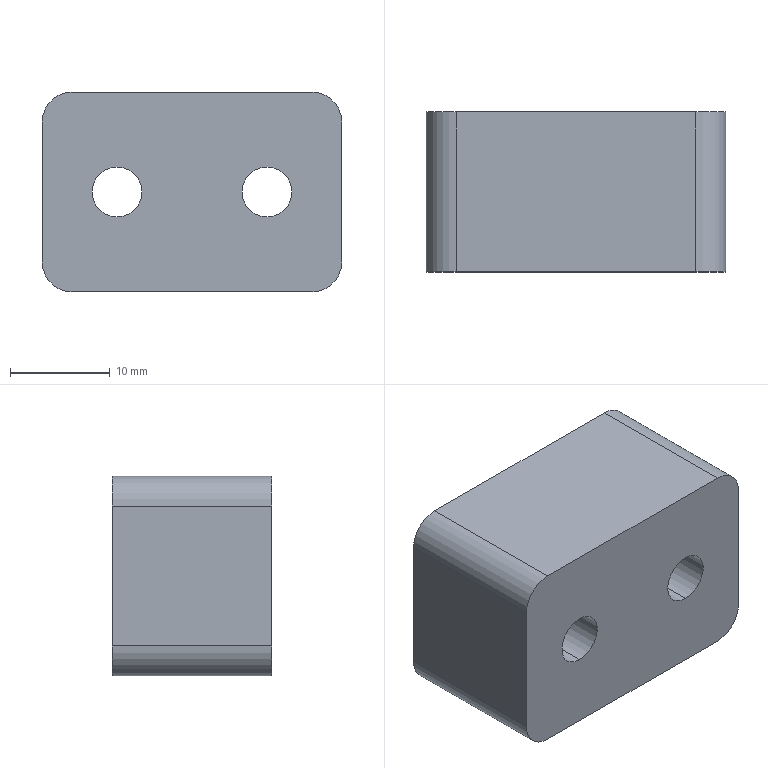Part | SolidWorks | features BaseBody 1 | 1 solid | 14 faces | box 30 x 16 x 20 mm | volume 8848 mm3 | cylinder 8 | plane 6 | commonest cylinder face diameters 5 x4 6 x4
STEP:
#1=CARTESIAN_POINT('',(-7.5,0.,-2.5));
#2=VERTEX_POINT('',#1);
#3=CARTESIAN_POINT('',(-7.5,0.,2.5));
#4=VERTEX_POINT('',#3);
#5=CARTESIAN_POINT('',(-7.5,0.,0.));
#6=DIRECTION('',(0.,1.,0.));
#7=DIRECTION('',(0.,0.,1.));
#8=AXIS2_PLACEMENT_3D('',#5,#6,#7);
#9=CIRCLE('',#8,2.5);
#10=EDGE_CURVE('',#2,#4,#9,.T.);
#11=ORIENTED_EDGE('',*,*,#10,.F.);
#12=CARTESIAN_POINT('',(-7.5,16.,-2.5));
#13=VERTEX_POINT('',#12);
#14=CARTESIAN_POINT('',(-7.5,0.,-2.5));
#15=DIRECTION('',(0.,1.,0.));
#16=VECTOR('',#15,1000.);
#17=LINE('',#14,#16);
#18=EDGE_CURVE('',#2,#13,#17,.T.);
#19=ORIENTED_EDGE('',*,*,#18,.T.);
#20=CARTESIAN_POINT('',(-7.5,16.,2.5));
#21=VERTEX_POINT('',#20);
#22=CARTESIAN_POINT('',(-7.5,16.,0.));
#23=DIRECTION('',(0.,-1.,0.));
#24=DIRECTION('',(0.,0.,1.));
#25=AXIS2_PLACEMENT_3D('',#22,#23,#24);
#26=CIRCLE('',#25,2.5);
#27=EDGE_CURVE('',#21,#13,#26,.T.);
#28=ORIENTED_EDGE('',*,*,#27,.F.);
#29=CARTESIAN_POINT('',(-7.5,0.,2.5));
#30=DIRECTION('',(0.,1.,0.));
#31=VECTOR('',#30,1000.);
#32=LINE('',#29,#31);
#33=EDGE_CURVE('',#4,#21,#32,.T.);
#34=ORIENTED_EDGE('',*,*,#33,.F.);
#35=EDGE_LOOP('',(#11,#19,#28,#34));
#36=FACE_OUTER_BOUND('',#35,.T.);
#37=CARTESIAN_POINT('',(-7.5,0.,0.));
#38=DIRECTION('',(0.,1.,0.));
#39=DIRECTION('',(0.,0.,1.));
#40=AXIS2_PLACEMENT_3D('',#37,#38,#39);
#41=CYLINDRICAL_SURFACE('',#40,2.5);
#42=ADVANCED_FACE('',(#36),#41,.F.);
#43=CARTESIAN_POINT('',(7.5,0.,-2.5));
#44=VERTEX_POINT('',#43);
#45=CARTESIAN_POINT('',(7.5,0.,2.5));
#46=VERTEX_POINT('',#45);
#47=CARTESIAN_POINT('',(7.5,0.,0.));
#48=DIRECTION('',(0.,1.,0.));
#49=DIRECTION('',(0.,0.,1.));
#50=AXIS2_PLACEMENT_3D('',#47,#48,#49);
#51=CIRCLE('',#50,2.5);
#52=EDGE_CURVE('',#44,#46,#51,.T.);
#53=ORIENTED_EDGE('',*,*,#52,.F.);
#54=CARTESIAN_POINT('',(7.5,16.,-2.5));
#55=VERTEX_POINT('',#54);
#56=CARTESIAN_POINT('',(7.5,0.,-2.5));
#57=DIRECTION('',(0.,1.,0.));
#58=VECTOR('',#57,1000.);
#59=LINE('',#56,#58);
#60=EDGE_CURVE('',#44,#55,#59,.T.);
#61=ORIENTED_EDGE('',*,*,#60,.T.);
#62=CARTESIAN_POINT('',(7.5,16.,2.5));
#63=VERTEX_POINT('',#62);
#64=CARTESIAN_POINT('',(7.5,16.,0.));
#65=DIRECTION('',(0.,-1.,0.));
#66=DIRECTION('',(0.,0.,1.));
#67=AXIS2_PLACEMENT_3D('',#64,#65,#66);
#68=CIRCLE('',#67,2.5);
#69=EDGE_CURVE('',#63,#55,#68,.T.);
#70=ORIENTED_EDGE('',*,*,#69,.F.);
#71=CARTESIAN_POINT('',(7.5,0.,2.5));
#72=DIRECTION('',(0.,1.,0.));
#73=VECTOR('',#72,1000.);
#74=LINE('',#71,#73);
#75=EDGE_CURVE('',#46,#63,#74,.T.);
#76=ORIENTED_EDGE('',*,*,#75,.F.);
#77=EDGE_LOOP('',(#53,#61,#70,#76));
#78=FACE_OUTER_BOUND('',#77,.T.);
#79=CARTESIAN_POINT('',(7.5,0.,0.));
#80=DIRECTION('',(0.,1.,0.));
#81=DIRECTION('',(0.,0.,1.));
#82=AXIS2_PLACEMENT_3D('',#79,#80,#81);
#83=CYLINDRICAL_SURFACE('',#82,2.5);
#84=ADVANCED_FACE('',(#78),#83,.F.);
#85=CARTESIAN_POINT('',(15.,0.,-7.));
#86=VERTEX_POINT('',#85);
#87=CARTESIAN_POINT('',(15.,0.,7.));
#88=VERTEX_POINT('',#87);
#89=CARTESIAN_POINT('',(15.,0.,0.));
#90=DIRECTION('',(0.,0.,1.));
#91=VECTOR('',#90,1000.);
#92=LINE('',#89,#91);
#93=EDGE_CURVE('',#86,#88,#92,.T.);
#94=ORIENTED_EDGE('',*,*,#93,.T.);
#95=CARTESIAN_POINT('',(12.,0.,10.));
#96=VERTEX_POINT('',#95);
#97=CARTESIAN_POINT('',(12.,0.,7.));
#98=DIRECTION('',(0.,-1.,0.));
#99=DIRECTION('',(0.,0.,-1.));
#100=AXIS2_PLACEMENT_3D('',#97,#98,#99);
#101=CIRCLE('',#100,3.);
#102=EDGE_CURVE('',#88,#96,#101,.T.);
#103=ORIENTED_EDGE('',*,*,#102,.T.);
#104=CARTESIAN_POINT('',(-12.,0.,10.));
#105=VERTEX_POINT('',#104);
#106=CARTESIAN_POINT('',(0.,0.,10.));
#107=DIRECTION('',(-1.,0.,0.));
#108=VECTOR('',#107,1000.);
#109=LINE('',#106,#108);
#110=EDGE_CURVE('',#96,#105,#109,.T.);
#111=ORIENTED_EDGE('',*,*,#110,.T.);
#112=CARTESIAN_POINT('',(-15.,0.,7.));
#113=VERTEX_POINT('',#112);
#114=CARTESIAN_POINT('',(-12.,0.,7.));
#115=DIRECTION('',(0.,-1.,0.));
#116=DIRECTION('',(0.,0.,-1.));
#117=AXIS2_PLACEMENT_3D('',#114,#115,#116);
#118=CIRCLE('',#117,3.);
#119=EDGE_CURVE('',#105,#113,#118,.T.);
#120=ORIENTED_EDGE('',*,*,#119,.T.);
#121=CARTESIAN_POINT('',(-15.,0.,-7.));
#122=VERTEX_POINT('',#121);
#123=CARTESIAN_POINT('',(-15.,0.,0.));
#124=DIRECTION('',(0.,0.,-1.));
#125=VECTOR('',#124,1000.);
#126=LINE('',#123,#125);
#127=EDGE_CURVE('',#113,#122,#126,.T.);
#128=ORIENTED_EDGE('',*,*,#127,.T.);
#129=CARTESIAN_POINT('',(-12.,0.,-10.));
#130=VERTEX_POINT('',#129);
#131=CARTESIAN_POINT('',(-12.,0.,-7.));
#132=DIRECTION('',(0.,-1.,0.));
#133=DIRECTION('',(0.,0.,-1.));
#134=AXIS2_PLACEMENT_3D('',#131,#132,#133);
#135=CIRCLE('',#134,3.);
#136=EDGE_CURVE('',#122,#130,#135,.T.);
#137=ORIENTED_EDGE('',*,*,#136,.T.);
#138=CARTESIAN_POINT('',(12.,0.,-10.));
#139=VERTEX_POINT('',#138);
#140=CARTESIAN_POINT('',(0.,0.,-10.));
#141=DIRECTION('',(1.,0.,0.));
#142=VECTOR('',#141,1000.);
#143=LINE('',#140,#142);
#144=EDGE_CURVE('',#130,#139,#143,.T.);
#145=ORIENTED_EDGE('',*,*,#144,.T.);
#146=CARTESIAN_POINT('',(12.,0.,-7.));
#147=DIRECTION('',(0.,-1.,0.));
#148=DIRECTION('',(0.,0.,-1.));
#149=AXIS2_PLACEMENT_3D('',#146,#147,#148);
#150=CIRCLE('',#149,3.);
#151=EDGE_CURVE('',#139,#86,#150,.T.);
#152=ORIENTED_EDGE('',*,*,#151,.T.);
#153=EDGE_LOOP('',(#94,#103,#111,#120,#128,#137,#145,#152));
#154=FACE_OUTER_BOUND('',#153,.T.);
#155=CARTESIAN_POINT('',(-7.5,0.,0.));
#156=DIRECTION('',(0.,1.,0.));
#157=DIRECTION('',(0.,0.,1.));
#158=AXIS2_PLACEMENT_3D('',#155,#156,#157);
#159=CIRCLE('',#158,2.5);
#160=EDGE_CURVE('',#4,#2,#159,.T.);
#161=ORIENTED_EDGE('',*,*,#160,.T.);
#162=ORIENTED_EDGE('',*,*,#10,.T.);
#163=EDGE_LOOP('',(#161,#162));
#164=FACE_BOUND('',#163,.T.);
#165=CARTESIAN_POINT('',(7.5,0.,0.));
#166=DIRECTION('',(0.,1.,0.));
#167=DIRECTION('',(0.,0.,1.));
#168=AXIS2_PLACEMENT_3D('',#165,#166,#167);
#169=CIRCLE('',#168,2.5);
#170=EDGE_CURVE('',#46,#44,#169,.T.);
#171=ORIENTED_EDGE('',*,*,#170,.T.);
#172=ORIENTED_EDGE('',*,*,#52,.T.);
#173=EDGE_LOOP('',(#171,#172));
#174=FACE_BOUND('',#173,.T.);
#175=CARTESIAN_POINT('',(0.,0.,0.));
#176=DIRECTION('',(0.,-1.,0.));
#177=DIRECTION('',(0.,0.,-1.));
#178=AXIS2_PLACEMENT_3D('',#175,#176,#177);
#179=PLANE('',#178);
#180=ADVANCED_FACE('',(#154,#164,#174),#179,.T.);
#181=ORIENTED_EDGE('',*,*,#102,.F.);
#182=CARTESIAN_POINT('',(15.,16.,7.));
#183=VERTEX_POINT('',#182);
#184=CARTESIAN_POINT('',(15.,16.,7.));
#185=DIRECTION('',(0.,1.,0.));
#186=VECTOR('',#185,1000.);
#187=LINE('',#184,#186);
#188=EDGE_CURVE('',#88,#183,#187,.T.);
#189=ORIENTED_EDGE('',*,*,#188,.T.);
#190=CARTESIAN_POINT('',(12.,16.,10.));
#191=VERTEX_POINT('',#190);
#192=CARTESIAN_POINT('',(12.,16.,7.));
#193=DIRECTION('',(0.,-1.,0.));
#194=DIRECTION('',(0.,0.,-1.));
#195=AXIS2_PLACEMENT_3D('',#192,#193,#194);
#196=CIRCLE('',#195,3.);
#197=EDGE_CURVE('',#183,#191,#196,.T.);
#198=ORIENTED_EDGE('',*,*,#197,.T.);
#199=CARTESIAN_POINT('',(12.,16.,10.));
#200=DIRECTION('',(0.,-1.,0.));
#201=VECTOR('',#200,1000.);
#202=LINE('',#199,#201);
#203=EDGE_CURVE('',#191,#96,#202,.T.);
#204=ORIENTED_EDGE('',*,*,#203,.T.);
#205=EDGE_LOOP('',(#181,#189,#198,#204));
#206=FACE_OUTER_BOUND('',#205,.T.);
#207=CARTESIAN_POINT('',(12.,16.,7.));
#208=DIRECTION('',(0.,-1.,0.));
#209=DIRECTION('',(0.,0.,-1.));
#210=AXIS2_PLACEMENT_3D('',#207,#208,#209);
#211=CYLINDRICAL_SURFACE('',#210,3.);
#212=ADVANCED_FACE('',(#206),#211,.T.);
#213=CARTESIAN_POINT('',(15.,16.,-7.));
#214=VERTEX_POINT('',#213);
#215=CARTESIAN_POINT('',(15.,16.,-7.));
#216=DIRECTION('',(0.,-1.,0.));
#217=VECTOR('',#216,1000.);
#218=LINE('',#215,#217);
#219=EDGE_CURVE('',#214,#86,#218,.T.);
#220=ORIENTED_EDGE('',*,*,#219,.F.);
#221=CARTESIAN_POINT('',(15.,16.,10.));
#222=DIRECTION('',(0.,0.,-1.));
#223=VECTOR('',#222,1000.);
#224=LINE('',#221,#223);
#225=EDGE_CURVE('',#183,#214,#224,.T.);
#226=ORIENTED_EDGE('',*,*,#225,.F.);
#227=ORIENTED_EDGE('',*,*,#188,.F.);
#228=ORIENTED_EDGE('',*,*,#93,.F.);
#229=EDGE_LOOP('',(#220,#226,#227,#228));
#230=FACE_OUTER_BOUND('',#229,.T.);
#231=CARTESIAN_POINT('',(15.,16.,10.));
#232=DIRECTION('',(-1.,0.,0.));
#233=DIRECTION('',(0.,0.,1.));
#234=AXIS2_PLACEMENT_3D('',#231,#232,#233);
#235=PLANE('',#234);
#236=ADVANCED_FACE('',(#230),#235,.F.);
#237=ORIENTED_EDGE('',*,*,#151,.F.);
#238=CARTESIAN_POINT('',(12.,16.,-10.));
#239=VERTEX_POINT('',#238);
#240=CARTESIAN_POINT('',(12.,16.,-10.));
#241=DIRECTION('',(0.,1.,0.));
#242=VECTOR('',#241,1000.);
#243=LINE('',#240,#242);
#244=EDGE_CURVE('',#139,#239,#243,.T.);
#245=ORIENTED_EDGE('',*,*,#244,.T.);
#246=CARTESIAN_POINT('',(12.,16.,-7.));
#247=DIRECTION('',(0.,-1.,0.));
#248=DIRECTION('',(0.,0.,-1.));
#249=AXIS2_PLACEMENT_3D('',#246,#247,#248);
#250=CIRCLE('',#249,3.);
#251=EDGE_CURVE('',#239,#214,#250,.T.);
#252=ORIENTED_EDGE('',*,*,#251,.T.);
#253=ORIENTED_EDGE('',*,*,#219,.T.);
#254=EDGE_LOOP('',(#237,#245,#252,#253));
#255=FACE_OUTER_BOUND('',#254,.T.);
#256=CARTESIAN_POINT('',(12.,16.,-7.));
#257=DIRECTION('',(0.,-1.,0.));
#258=DIRECTION('',(0.,0.,-1.));
#259=AXIS2_PLACEMENT_3D('',#256,#257,#258);
#260=CYLINDRICAL_SURFACE('',#259,3.);
#261=ADVANCED_FACE('',(#255),#260,.T.);
#262=CARTESIAN_POINT('',(-12.,16.,-10.));
#263=VERTEX_POINT('',#262);
#264=CARTESIAN_POINT('',(-12.,16.,-10.));
#265=DIRECTION('',(0.,-1.,0.));
#266=VECTOR('',#265,1000.);
#267=LINE('',#264,#266);
#268=EDGE_CURVE('',#263,#130,#267,.T.);
#269=ORIENTED_EDGE('',*,*,#268,.F.);
#270=CARTESIAN_POINT('',(-15.,16.,-10.));
#271=DIRECTION('',(-1.,0.,0.));
#272=VECTOR('',#271,1000.);
#273=LINE('',#270,#272);
#274=EDGE_CURVE('',#239,#263,#273,.T.);
#275=ORIENTED_EDGE('',*,*,#274,.F.);
#276=ORIENTED_EDGE('',*,*,#244,.F.);
#277=ORIENTED_EDGE('',*,*,#144,.F.);
#278=EDGE_LOOP('',(#269,#275,#276,#277));
#279=FACE_OUTER_BOUND('',#278,.T.);
#280=CARTESIAN_POINT('',(-15.,16.,-10.));
#281=DIRECTION('',(0.,0.,1.));
#282=DIRECTION('',(1.,0.,0.));
#283=AXIS2_PLACEMENT_3D('',#280,#281,#282);
#284=PLANE('',#283);
#285=ADVANCED_FACE('',(#279),#284,.F.);
#286=ORIENTED_EDGE('',*,*,#136,.F.);
#287=CARTESIAN_POINT('',(-15.,16.,-7.));
#288=VERTEX_POINT('',#287);
#289=CARTESIAN_POINT('',(-15.,16.,-7.));
#290=DIRECTION('',(0.,1.,0.));
#291=VECTOR('',#290,1000.);
#292=LINE('',#289,#291);
#293=EDGE_CURVE('',#122,#288,#292,.T.);
#294=ORIENTED_EDGE('',*,*,#293,.T.);
#295=CARTESIAN_POINT('',(-12.,16.,-7.));
#296=DIRECTION('',(0.,-1.,0.));
#297=DIRECTION('',(0.,0.,-1.));
#298=AXIS2_PLACEMENT_3D('',#295,#296,#297);
#299=CIRCLE('',#298,3.);
#300=EDGE_CURVE('',#288,#263,#299,.T.);
#301=ORIENTED_EDGE('',*,*,#300,.T.);
#302=ORIENTED_EDGE('',*,*,#268,.T.);
#303=EDGE_LOOP('',(#286,#294,#301,#302));
#304=FACE_OUTER_BOUND('',#303,.T.);
#305=CARTESIAN_POINT('',(-12.,16.,-7.));
#306=DIRECTION('',(0.,-1.,0.));
#307=DIRECTION('',(0.,0.,-1.));
#308=AXIS2_PLACEMENT_3D('',#305,#306,#307);
#309=CYLINDRICAL_SURFACE('',#308,3.);
#310=ADVANCED_FACE('',(#304),#309,.T.);
#311=CARTESIAN_POINT('',(-15.,16.,7.));
#312=VERTEX_POINT('',#311);
#313=CARTESIAN_POINT('',(-15.,16.,7.));
#314=DIRECTION('',(0.,-1.,0.));
#315=VECTOR('',#314,1000.);
#316=LINE('',#313,#315);
#317=EDGE_CURVE('',#312,#113,#316,.T.);
#318=ORIENTED_EDGE('',*,*,#317,.F.);
#319=CARTESIAN_POINT('',(-15.,16.,10.));
#320=DIRECTION('',(0.,0.,1.));
#321=VECTOR('',#320,1000.);
#322=LINE('',#319,#321);
#323=EDGE_CURVE('',#288,#312,#322,.T.);
#324=ORIENTED_EDGE('',*,*,#323,.F.);
#325=ORIENTED_EDGE('',*,*,#293,.F.);
#326=ORIENTED_EDGE('',*,*,#127,.F.);
#327=EDGE_LOOP('',(#318,#324,#325,#326));
#328=FACE_OUTER_BOUND('',#327,.T.);
#329=CARTESIAN_POINT('',(-15.,16.,10.));
#330=DIRECTION('',(1.,0.,0.));
#331=DIRECTION('',(0.,0.,-1.));
#332=AXIS2_PLACEMENT_3D('',#329,#330,#331);
#333=PLANE('',#332);
#334=ADVANCED_FACE('',(#328),#333,.F.);
#335=ORIENTED_EDGE('',*,*,#119,.F.);
#336=CARTESIAN_POINT('',(-12.,16.,10.));
#337=VERTEX_POINT('',#336);
#338=CARTESIAN_POINT('',(-12.,16.,10.));
#339=DIRECTION('',(0.,1.,0.));
#340=VECTOR('',#339,1000.);
#341=LINE('',#338,#340);
#342=EDGE_CURVE('',#105,#337,#341,.T.);
#343=ORIENTED_EDGE('',*,*,#342,.T.);
#344=CARTESIAN_POINT('',(-12.,16.,7.));
#345=DIRECTION('',(0.,-1.,0.));
#346=DIRECTION('',(0.,0.,-1.));
#347=AXIS2_PLACEMENT_3D('',#344,#345,#346);
#348=CIRCLE('',#347,3.);
#349=EDGE_CURVE('',#337,#312,#348,.T.);
#350=ORIENTED_EDGE('',*,*,#349,.T.);
#351=ORIENTED_EDGE('',*,*,#317,.T.);
#352=EDGE_LOOP('',(#335,#343,#350,#351));
#353=FACE_OUTER_BOUND('',#352,.T.);
#354=CARTESIAN_POINT('',(-12.,16.,7.));
#355=DIRECTION('',(0.,-1.,0.));
#356=DIRECTION('',(0.,0.,-1.));
#357=AXIS2_PLACEMENT_3D('',#354,#355,#356);
#358=CYLINDRICAL_SURFACE('',#357,3.);
#359=ADVANCED_FACE('',(#353),#358,.T.);
#360=ORIENTED_EDGE('',*,*,#342,.F.);
#361=ORIENTED_EDGE('',*,*,#110,.F.);
#362=ORIENTED_EDGE('',*,*,#203,.F.);
#363=CARTESIAN_POINT('',(-15.,16.,10.));
#364=DIRECTION('',(1.,0.,0.));
#365=VECTOR('',#364,1000.);
#366=LINE('',#363,#365);
#367=EDGE_CURVE('',#337,#191,#366,.T.);
#368=ORIENTED_EDGE('',*,*,#367,.F.);
#369=EDGE_LOOP('',(#360,#361,#362,#368));
#370=FACE_OUTER_BOUND('',#369,.T.);
#371=CARTESIAN_POINT('',(-15.,16.,10.));
#372=DIRECTION('',(0.,0.,-1.));
#373=DIRECTION('',(-1.,0.,0.));
#374=AXIS2_PLACEMENT_3D('',#371,#372,#373);
#375=PLANE('',#374);
#376=ADVANCED_FACE('',(#370),#375,.F.);
#377=ORIENTED_EDGE('',*,*,#18,.F.);
#378=ORIENTED_EDGE('',*,*,#160,.F.);
#379=ORIENTED_EDGE('',*,*,#33,.T.);
#380=CARTESIAN_POINT('',(-7.5,16.,0.));
#381=DIRECTION('',(0.,-1.,0.));
#382=DIRECTION('',(0.,0.,1.));
#383=AXIS2_PLACEMENT_3D('',#380,#381,#382);
#384=CIRCLE('',#383,2.5);
#385=EDGE_CURVE('',#13,#21,#384,.T.);
#386=ORIENTED_EDGE('',*,*,#385,.F.);
#387=EDGE_LOOP('',(#377,#378,#379,#386));
#388=FACE_OUTER_BOUND('',#387,.T.);
#389=CARTESIAN_POINT('',(-7.5,0.,0.));
#390=DIRECTION('',(0.,1.,0.));
#391=DIRECTION('',(0.,0.,1.));
#392=AXIS2_PLACEMENT_3D('',#389,#390,#391);
#393=CYLINDRICAL_SURFACE('',#392,2.5);
#394=ADVANCED_FACE('',(#388),#393,.F.);
#395=ORIENTED_EDGE('',*,*,#60,.F.);
#396=ORIENTED_EDGE('',*,*,#170,.F.);
#397=ORIENTED_EDGE('',*,*,#75,.T.);
#398=CARTESIAN_POINT('',(7.5,16.,0.));
#399=DIRECTION('',(0.,-1.,0.));
#400=DIRECTION('',(0.,0.,1.));
#401=AXIS2_PLACEMENT_3D('',#398,#399,#400);
#402=CIRCLE('',#401,2.5);
#403=EDGE_CURVE('',#55,#63,#402,.T.);
#404=ORIENTED_EDGE('',*,*,#403,.F.);
#405=EDGE_LOOP('',(#395,#396,#397,#404));
#406=FACE_OUTER_BOUND('',#405,.T.);
#407=CARTESIAN_POINT('',(7.5,0.,0.));
#408=DIRECTION('',(0.,1.,0.));
#409=DIRECTION('',(0.,0.,1.));
#410=AXIS2_PLACEMENT_3D('',#407,#408,#409);
#411=CYLINDRICAL_SURFACE('',#410,2.5);
#412=ADVANCED_FACE('',(#406),#411,.F.);
#413=ORIENTED_EDGE('',*,*,#349,.F.);
#414=ORIENTED_EDGE('',*,*,#367,.T.);
#415=ORIENTED_EDGE('',*,*,#197,.F.);
#416=ORIENTED_EDGE('',*,*,#225,.T.);
#417=ORIENTED_EDGE('',*,*,#251,.F.);
#418=ORIENTED_EDGE('',*,*,#274,.T.);
#419=ORIENTED_EDGE('',*,*,#300,.F.);
#420=ORIENTED_EDGE('',*,*,#323,.T.);
#421=EDGE_LOOP('',(#413,#414,#415,#416,#417,#418,#419,#420));
#422=FACE_OUTER_BOUND('',#421,.T.);
#423=ORIENTED_EDGE('',*,*,#27,.T.);
#424=ORIENTED_EDGE('',*,*,#385,.T.);
#425=EDGE_LOOP('',(#423,#424));
#426=FACE_BOUND('',#425,.T.);
#427=ORIENTED_EDGE('',*,*,#69,.T.);
#428=ORIENTED_EDGE('',*,*,#403,.T.);
#429=EDGE_LOOP('',(#427,#428));
#430=FACE_BOUND('',#429,.T.);
#431=CARTESIAN_POINT('',(0.,16.,0.));
#432=DIRECTION('',(0.,-1.,0.));
#433=DIRECTION('',(0.,0.,-1.));
#434=AXIS2_PLACEMENT_3D('',#431,#432,#433);
#435=PLANE('',#434);
#436=ADVANCED_FACE('',(#422,#426,#430),#435,.F.);
#437=CLOSED_SHELL('',(#42,#84,#180,#212,#236,#261,#285,#310,#334,#359,#376,#394,#412,#436));
#438=MANIFOLD_SOLID_BREP('',#437);
#439=CARTESIAN_POINT('',(0.,0.,0.));
#440=DIRECTION('',(0.,0.,1.));
#441=DIRECTION('',(1.,0.,0.));
#442=AXIS2_PLACEMENT_3D('',#439,#440,#441);
#443=(LENGTH_UNIT()NAMED_UNIT(*)SI_UNIT(.MILLI.,.METRE.));
#444=UNCERTAINTY_MEASURE_WITH_UNIT(LENGTH_MEASURE(0.00001),#443,'','');
#445=(NAMED_UNIT(*)PLANE_ANGLE_UNIT()SI_UNIT($,.RADIAN.));
#446=(NAMED_UNIT(*)SI_UNIT($,.STERADIAN.)SOLID_ANGLE_UNIT());
#447=(GEOMETRIC_REPRESENTATION_CONTEXT(3)GLOBAL_UNCERTAINTY_ASSIGNED_CONTEXT((#444))GLOBAL_UNIT_ASSIGNED_CONTEXT((#443,#445,#446))REPRESENTATION_CONTEXT('',''));
#448=ADVANCED_BREP_SHAPE_REPRESENTATION('',(#438,#442),#447);